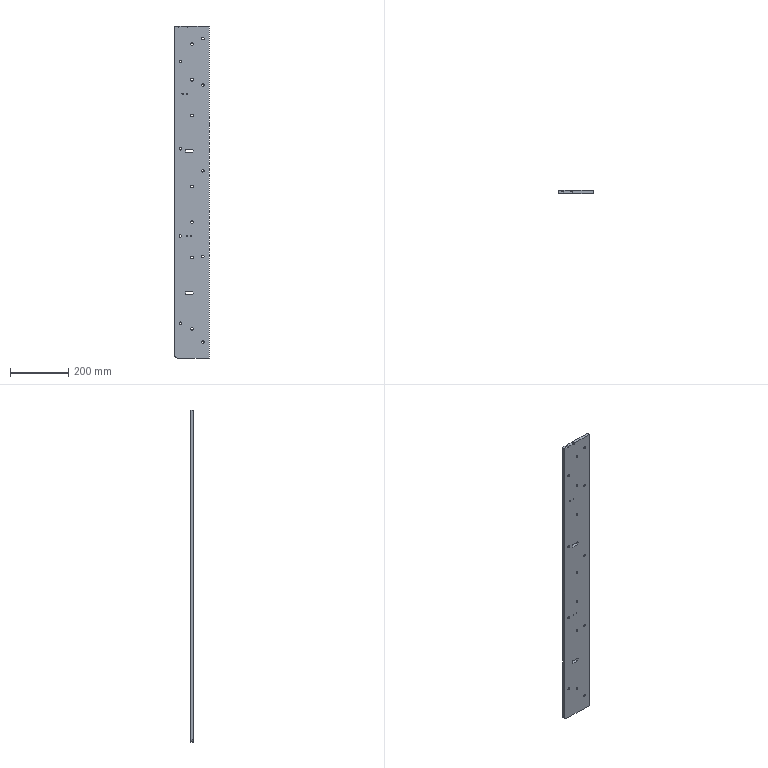Part | STEP file | 1 solid | 67 faces | box 120 x 10 x 1143 mm | volume 1355255 mm3 | cylinder 49 | plane 18 | commonest cylinder face diameters 9 x14 8.4 x10 4.2 x8 8.5 x8 2 x4 7 x4